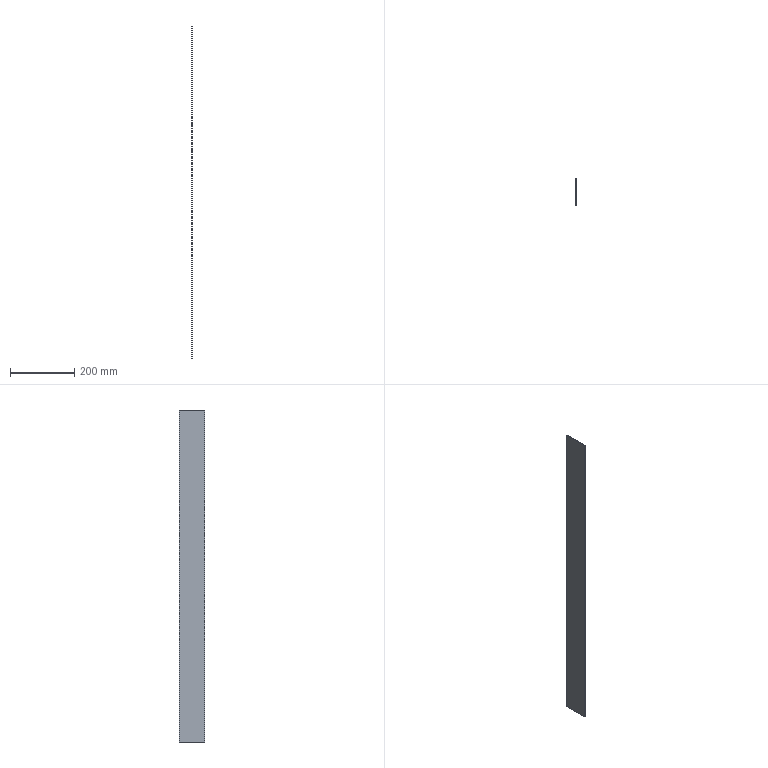Part | SolidWorks | 1 solid | 6 faces | box 1.5 x 80 x 1030 mm | volume 123600 mm3 | plane 6
STEP:
#1=CARTESIAN_POINT('',(0.,40.,515.));
#2=VERTEX_POINT('',#1);
#3=CARTESIAN_POINT('',(0.,-40.,515.));
#4=VERTEX_POINT('',#3);
#5=CARTESIAN_POINT('',(0.,-40.,515.));
#6=DIRECTION('',(0.,-1.,0.));
#7=VECTOR('',#6,1000.);
#8=LINE('',#5,#7);
#9=EDGE_CURVE('',#2,#4,#8,.T.);
#10=ORIENTED_EDGE('',*,*,#9,.F.);
#11=CARTESIAN_POINT('',(-1.5,40.,515.));
#12=VERTEX_POINT('',#11);
#13=CARTESIAN_POINT('',(-1.5,40.,515.));
#14=DIRECTION('',(1.,0.,0.));
#15=VECTOR('',#14,1000.);
#16=LINE('',#13,#15);
#17=EDGE_CURVE('',#12,#2,#16,.T.);
#18=ORIENTED_EDGE('',*,*,#17,.F.);
#19=CARTESIAN_POINT('',(-1.5,-40.,515.));
#20=VERTEX_POINT('',#19);
#21=CARTESIAN_POINT('',(-1.5,-40.,515.));
#22=DIRECTION('',(0.,-1.,0.));
#23=VECTOR('',#22,1000.);
#24=LINE('',#21,#23);
#25=EDGE_CURVE('',#12,#20,#24,.T.);
#26=ORIENTED_EDGE('',*,*,#25,.T.);
#27=CARTESIAN_POINT('',(-1.5,-40.,515.));
#28=DIRECTION('',(1.,0.,0.));
#29=VECTOR('',#28,1000.);
#30=LINE('',#27,#29);
#31=EDGE_CURVE('',#20,#4,#30,.T.);
#32=ORIENTED_EDGE('',*,*,#31,.T.);
#33=EDGE_LOOP('',(#10,#18,#26,#32));
#34=FACE_OUTER_BOUND('',#33,.T.);
#35=CARTESIAN_POINT('',(-1.5,-40.,515.));
#36=DIRECTION('',(0.,0.,1.));
#37=DIRECTION('',(1.,0.,0.));
#38=AXIS2_PLACEMENT_3D('',#35,#36,#37);
#39=PLANE('',#38);
#40=ADVANCED_FACE('',(#34),#39,.T.);
#41=CARTESIAN_POINT('',(0.,40.,-515.));
#42=VERTEX_POINT('',#41);
#43=CARTESIAN_POINT('',(0.,40.,-515.));
#44=DIRECTION('',(0.,0.,1.));
#45=VECTOR('',#44,1000.);
#46=LINE('',#43,#45);
#47=EDGE_CURVE('',#42,#2,#46,.T.);
#48=ORIENTED_EDGE('',*,*,#47,.F.);
#49=CARTESIAN_POINT('',(-1.5,40.,-515.));
#50=VERTEX_POINT('',#49);
#51=CARTESIAN_POINT('',(-1.5,40.,-515.));
#52=DIRECTION('',(1.,0.,0.));
#53=VECTOR('',#52,1000.);
#54=LINE('',#51,#53);
#55=EDGE_CURVE('',#50,#42,#54,.T.);
#56=ORIENTED_EDGE('',*,*,#55,.F.);
#57=CARTESIAN_POINT('',(-1.5,40.,-515.));
#58=DIRECTION('',(0.,0.,1.));
#59=VECTOR('',#58,1000.);
#60=LINE('',#57,#59);
#61=EDGE_CURVE('',#50,#12,#60,.T.);
#62=ORIENTED_EDGE('',*,*,#61,.T.);
#63=ORIENTED_EDGE('',*,*,#17,.T.);
#64=EDGE_LOOP('',(#48,#56,#62,#63));
#65=FACE_OUTER_BOUND('',#64,.T.);
#66=CARTESIAN_POINT('',(-1.5,40.,-515.));
#67=DIRECTION('',(0.,1.,0.));
#68=DIRECTION('',(0.,0.,1.));
#69=AXIS2_PLACEMENT_3D('',#66,#67,#68);
#70=PLANE('',#69);
#71=ADVANCED_FACE('',(#65),#70,.T.);
#72=CARTESIAN_POINT('',(0.,-40.,-515.));
#73=VERTEX_POINT('',#72);
#74=CARTESIAN_POINT('',(0.,-40.,-515.));
#75=DIRECTION('',(0.,1.,0.));
#76=VECTOR('',#75,1000.);
#77=LINE('',#74,#76);
#78=EDGE_CURVE('',#73,#42,#77,.T.);
#79=ORIENTED_EDGE('',*,*,#78,.F.);
#80=CARTESIAN_POINT('',(-1.5,-40.,-515.));
#81=VERTEX_POINT('',#80);
#82=CARTESIAN_POINT('',(-1.5,-40.,-515.));
#83=DIRECTION('',(1.,0.,0.));
#84=VECTOR('',#83,1000.);
#85=LINE('',#82,#84);
#86=EDGE_CURVE('',#81,#73,#85,.T.);
#87=ORIENTED_EDGE('',*,*,#86,.F.);
#88=CARTESIAN_POINT('',(-1.5,-40.,-515.));
#89=DIRECTION('',(0.,1.,0.));
#90=VECTOR('',#89,1000.);
#91=LINE('',#88,#90);
#92=EDGE_CURVE('',#81,#50,#91,.T.);
#93=ORIENTED_EDGE('',*,*,#92,.T.);
#94=ORIENTED_EDGE('',*,*,#55,.T.);
#95=EDGE_LOOP('',(#79,#87,#93,#94));
#96=FACE_OUTER_BOUND('',#95,.T.);
#97=CARTESIAN_POINT('',(-1.5,-40.,-515.));
#98=DIRECTION('',(0.,0.,-1.));
#99=DIRECTION('',(-1.,0.,0.));
#100=AXIS2_PLACEMENT_3D('',#97,#98,#99);
#101=PLANE('',#100);
#102=ADVANCED_FACE('',(#96),#101,.T.);
#103=CARTESIAN_POINT('',(0.,-40.,-515.));
#104=DIRECTION('',(0.,0.,-1.));
#105=VECTOR('',#104,1000.);
#106=LINE('',#103,#105);
#107=EDGE_CURVE('',#4,#73,#106,.T.);
#108=ORIENTED_EDGE('',*,*,#107,.F.);
#109=ORIENTED_EDGE('',*,*,#31,.F.);
#110=CARTESIAN_POINT('',(-1.5,-40.,-515.));
#111=DIRECTION('',(0.,0.,-1.));
#112=VECTOR('',#111,1000.);
#113=LINE('',#110,#112);
#114=EDGE_CURVE('',#20,#81,#113,.T.);
#115=ORIENTED_EDGE('',*,*,#114,.T.);
#116=ORIENTED_EDGE('',*,*,#86,.T.);
#117=EDGE_LOOP('',(#108,#109,#115,#116));
#118=FACE_OUTER_BOUND('',#117,.T.);
#119=CARTESIAN_POINT('',(-1.5,-40.,-515.));
#120=DIRECTION('',(0.,-1.,0.));
#121=DIRECTION('',(0.,0.,-1.));
#122=AXIS2_PLACEMENT_3D('',#119,#120,#121);
#123=PLANE('',#122);
#124=ADVANCED_FACE('',(#118),#123,.T.);
#125=ORIENTED_EDGE('',*,*,#25,.F.);
#126=ORIENTED_EDGE('',*,*,#61,.F.);
#127=ORIENTED_EDGE('',*,*,#92,.F.);
#128=ORIENTED_EDGE('',*,*,#114,.F.);
#129=EDGE_LOOP('',(#125,#126,#127,#128));
#130=FACE_OUTER_BOUND('',#129,.T.);
#131=CARTESIAN_POINT('',(-1.5,0.,0.));
#132=DIRECTION('',(1.,0.,0.));
#133=DIRECTION('',(0.,0.,-1.));
#134=AXIS2_PLACEMENT_3D('',#131,#132,#133);
#135=PLANE('',#134);
#136=ADVANCED_FACE('',(#130),#135,.F.);
#137=ORIENTED_EDGE('',*,*,#9,.T.);
#138=ORIENTED_EDGE('',*,*,#107,.T.);
#139=ORIENTED_EDGE('',*,*,#78,.T.);
#140=ORIENTED_EDGE('',*,*,#47,.T.);
#141=EDGE_LOOP('',(#137,#138,#139,#140));
#142=FACE_OUTER_BOUND('',#141,.T.);
#143=CARTESIAN_POINT('',(0.,0.,0.));
#144=DIRECTION('',(1.,0.,0.));
#145=DIRECTION('',(0.,0.,-1.));
#146=AXIS2_PLACEMENT_3D('',#143,#144,#145);
#147=PLANE('',#146);
#148=ADVANCED_FACE('',(#142),#147,.T.);
#149=CLOSED_SHELL('',(#40,#71,#102,#124,#136,#148));
#150=MANIFOLD_SOLID_BREP('',#149);
#151=CARTESIAN_POINT('',(0.,0.,0.));
#152=DIRECTION('',(0.,0.,1.));
#153=DIRECTION('',(1.,0.,0.));
#154=AXIS2_PLACEMENT_3D('',#151,#152,#153);
#155=(LENGTH_UNIT()NAMED_UNIT(*)SI_UNIT(.MILLI.,.METRE.));
#156=UNCERTAINTY_MEASURE_WITH_UNIT(LENGTH_MEASURE(0.00001),#155,'','');
#157=(NAMED_UNIT(*)PLANE_ANGLE_UNIT()SI_UNIT($,.RADIAN.));
#158=(NAMED_UNIT(*)SI_UNIT($,.STERADIAN.)SOLID_ANGLE_UNIT());
#159=(GEOMETRIC_REPRESENTATION_CONTEXT(3)GLOBAL_UNCERTAINTY_ASSIGNED_CONTEXT((#156))GLOBAL_UNIT_ASSIGNED_CONTEXT((#155,#157,#158))REPRESENTATION_CONTEXT('',''));
#160=ADVANCED_BREP_SHAPE_REPRESENTATION('',(#150,#154),#159);